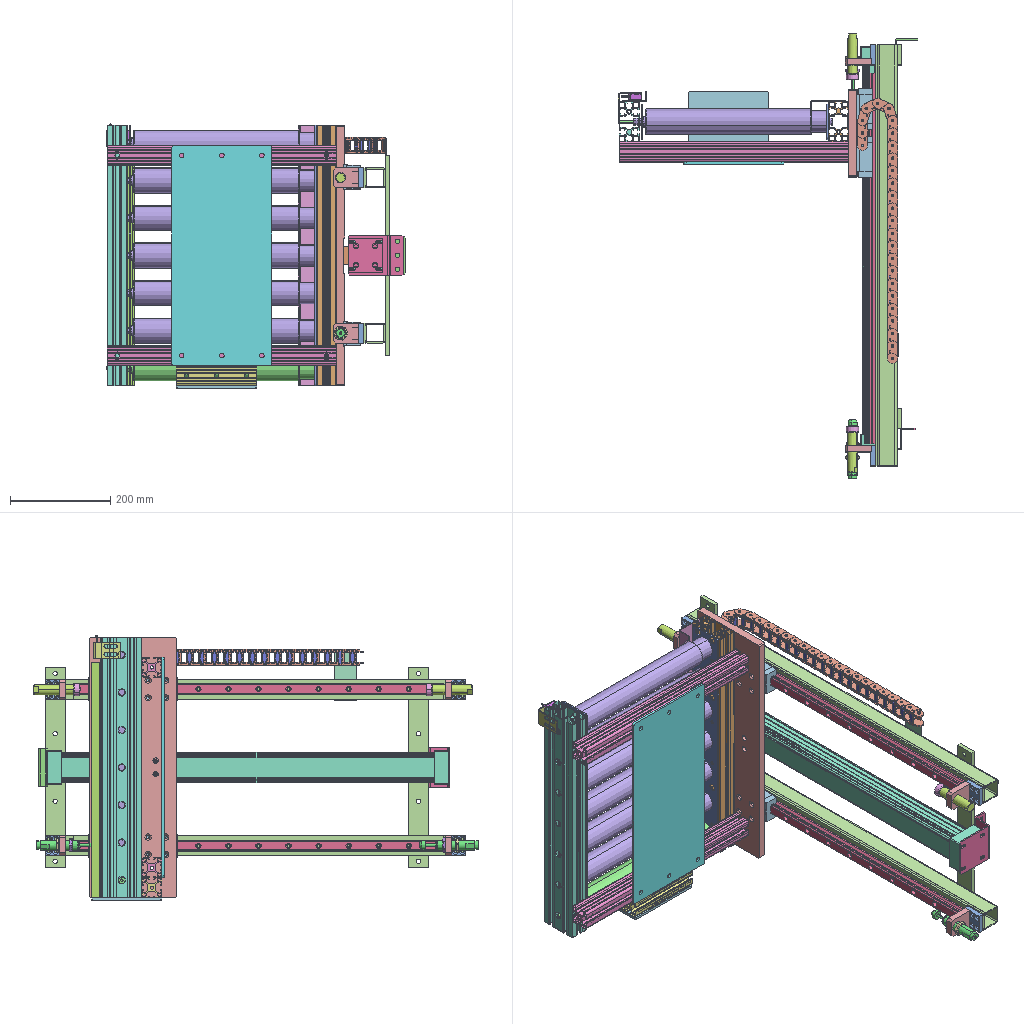Assembly | STEP file | 32 different items | 105 placed | box 598 x 888 x 528 mm
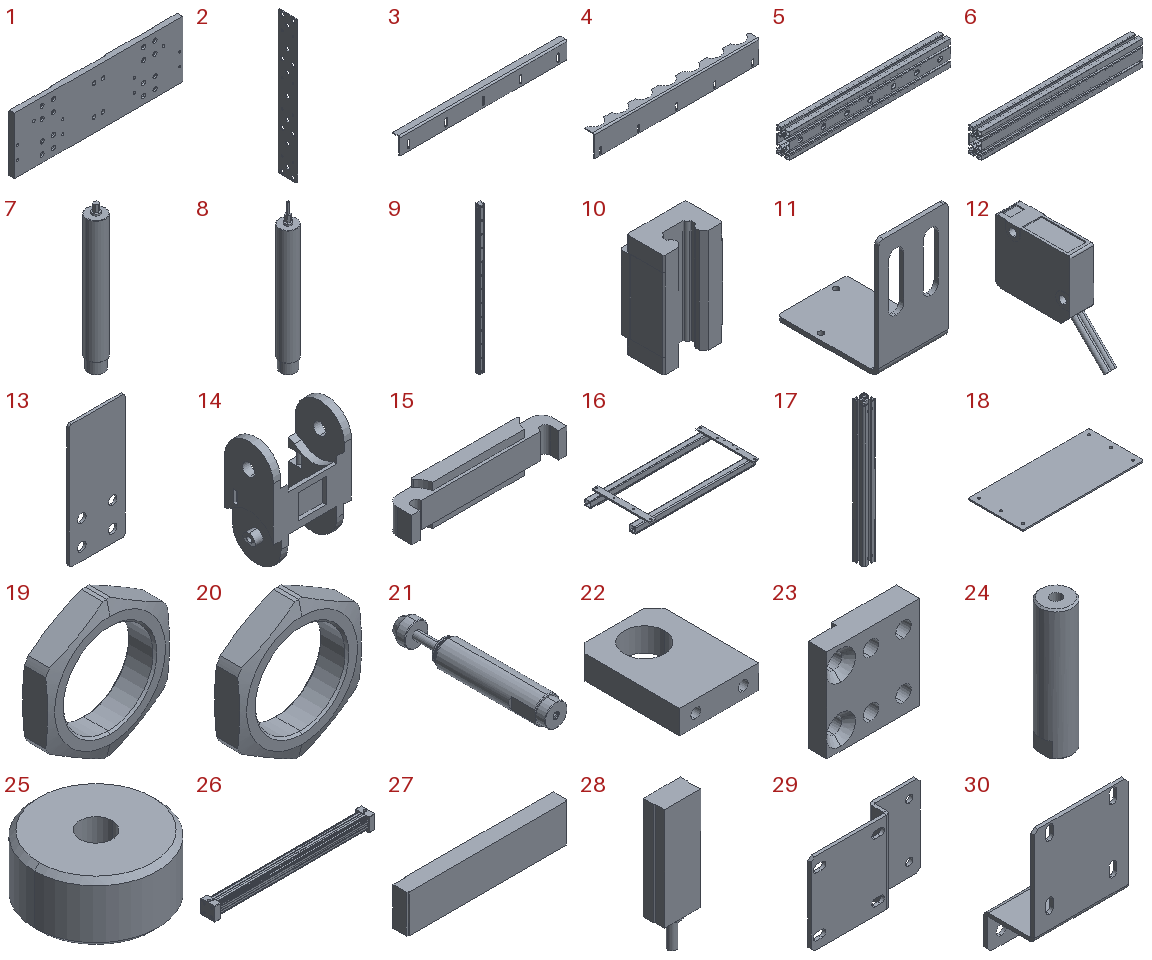Parts list (item | name | quantity | parent item | size | volume):
1 | - | x1 | - | 520 x 16 x 175 mm | 1376606 mm3
2 | - | x2 | - | 3 x 70 x 520 mm | 101913 mm3
3 | - | x1 | - | 470 x 20 x 48 mm | 59388 mm3
4 | - | x1 | - | 520 x 30 x 70 mm | 90245 mm3
5 | - | x1 | - | 520 x 40 x 80 mm | 382140 mm3
6 | - | x1 | - | 520 x 40 x 80 mm | 378549 mm3
7 | Unpowered Roller_Default | x6 | - | 50.6 x 50.6 x 396 mm | 712589 mm3
8 | Motorized Roller_Default | x1 | - | 50.6 x 50.6 x 426 mm | 713178 mm3
9 | HGH25 Rail | x2 | in HGH25CA2R740Z0 | 23 x 22 x 740 mm | 310065 mm3
10 | HGH25 Slider | x4 | in HGH25CA2R740Z0 | 48 x 34.5 x 82 mm | 100220 mm3
11 | - | x1 | - | 32 x 47 x 55 mm | 5577 mm3
12 | Proximity Switch | x1 | - | 10.4 x 45.161 x 39.591 mm | 8353 mm3
13 | - | x1 | - | 45 x 2 x 100 mm | 8685 mm3
14 | MHPU203_30c | x25 | in MHPU203_30_MHPU203-30 | 32 x 20 x 45 mm | 6087 mm3
15 | MHPU203_30f | x25 | in MHPU203_30_MHPU203-30 | 27.6 x 4.5 x 7.143 mm | 492.21 mm3
16 | - | x1 | - | 840 x 400 x 53 mm | 1080937 mm3
17 | - | x2 | - | 40 x 40 x 458 mm | 262404 mm3
18 | - | x1 | - | 440 x 200 x 5 mm | 437984 mm3
19 | ACA-2020-1 | x2 | in ACA-2020 | 26 x 6 x 29.132 mm | 1676 mm3
20 | ACA-2020-2 | x2 | in ACA-2020 | 26 x 6 x 29.132 mm | 1676 mm3
21 | ACA-2020-3 | x2 | in ACA-2020 | 20 x 118 x 20 mm | 28972 mm3
22 | - | x5 | - | 40 x 53 x 12 mm | 20571 mm3
23 | - | x5 | - | 40 x 10 x 40 mm | 12395 mm3
24 | - | x2 | - | 20 x 20 x 80 mm | 24015 mm3
25 | - | x2 | - | 25 x 25 x 12 mm | 5014 mm3
26 | HI_PRU40500b | x1 | in PRF40x500-S2_0_ | 800 x 69 x 69 mm | 2639652 mm3
27 | HI_PRF40500s | x1 | in PRF40x500-S2_0_ | 152 x 14 x 36 mm | 74599 mm3
28 | HI_S-CS-95 | x2 | in PRF40x500-S2_0_ | 10.9 x 7 x 39 mm | 1983 mm3
29 | - | x1 | - | 115 x 18 x 75 mm | 27777 mm3
30 | - | x1 | - | 80 x 43 x 110 mm | 34046 mm3
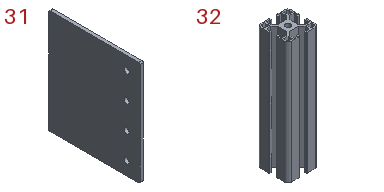31 | - | x1 | - | 5 x 140 x 160 mm | 110710 mm3
32 | - | x1 | - | 40 x 40 x 160 mm | 89766 mm3
Placements (level | parent | child | x y z in mm | rotation matrix by rows):
1 | subassembly 2 | subassembly 3 | -147.955 36.01 -80.412 | 0 1 0 0 0 -1 -1 0 0
1 | subassembly 2 | subassembly 4 | -187.955 71.51 -340.412 | -1 0 0 0 1 0 0 0 -1
1 | subassembly 2 | subassembly 4 | -558.455 71.51 -340.412 | -1 0 0 0 1 0 0 0 -1
1 | subassembly 2 | subassembly 5 | -598.455 98.51 129.588 | 0 0 1 0 1 0 -1 0 -0
1 | subassembly 2 | subassembly 6 | -154.455 100.51 179.588 | 0 0 -1 0 -1 0 -1 0 0
1 | subassembly 2 | subassembly 7 | -585.955 78.51 -340.412 | 0 1 0 0 0 1 1 0 0
1 | subassembly 2 | subassembly 8 | -167.955 38.51 -340.412 | 0 -1 0 0 0 -1 1 0 0
1 | subassembly 2 | Unpowered Roller_Default | -222.455 58.76 -230.412 | 0 0 -1 0.3439 -0.939 0 -0.939 -0.3439 0
1 | subassembly 2 | Unpowered Roller_Default | -222.455 58.76 144.588 | 0 0 -1 0.3439 -0.939 0 -0.939 -0.3439 0
1 | subassembly 2 | Unpowered Roller_Default | -222.455 58.76 69.588 | 0 0 -1 0.3439 -0.939 0 -0.939 -0.3439 0
1 | subassembly 2 | Unpowered Roller_Default | -222.455 58.76 -5.412 | 0 0 -1 0.3439 -0.939 0 -0.939 -0.3439 0
1 | subassembly 2 | Unpowered Roller_Default | -222.455 58.76 -80.412 | 0 0 -1 0.3439 -0.939 0 -0.939 -0.3439 0
1 | subassembly 2 | Unpowered Roller_Default | -222.455 58.76 -155.412 | 0 0 -1 0.3439 -0.939 0 -0.939 -0.3439 0
1 | subassembly 2 | Motorized Roller_Default | -222.455 58.361 -305.412 | 0 0 -1 0 1 0 1 0 0
1 | subassembly 2 | HGH25CA2R740Z0 | -108.387 -214.405 -232.617 | 0 -1 0 0 0 1 -1 0 -0
2 | HGH25CA2R740Z0 | HGH25 Rail | 4.046 -14.432 -225.0 | 1 0 0 0 1 0 0 0 1
2 | HGH25CA2R740Z0 | HGH25 Slider | 4.046 -14.432 297.916 | 1 0 0 0 1 0 0 0 1
2 | HGH25CA2R740Z0 | HGH25 Slider | 4.046 -14.432 202.916 | 1 0 0 0 1 0 0 0 1
1 | subassembly 2 | HGH25CA2R740Z0 | -108.387 -214.405 80.383 | 0 -1 0 0 0 1 -1 0 -0
2 | HGH25CA2R740Z0 | HGH25 Rail | 4.046 -14.432 -225.0 | 1 0 0 0 1 0 0 0 1
2 | HGH25CA2R740Z0 | HGH25 Slider | 4.046 -14.432 297.916 | 1 0 0 0 1 0 0 0 1
2 | HGH25CA2R740Z0 | HGH25 Slider | 4.046 -14.432 202.916 | 1 0 0 0 1 0 0 0 1
1 | subassembly 2 | subassembly 9 | -605.955 115.71 169.588 | 0 1 0 0 0 -1 -1 0 -0
1 | subassembly 2 | Proximity Switch | -563.955 108.51 145.388 | 0 0 1 -1 0 0 0 -1 0
1 | subassembly 2 | subassembly 10 | -47.955 -410.405 53.338 | 0 -1 0 1 0 0 0 0 1
1 | subassembly 2 | MHPU203_30_MHPU203-30 | -119.955 58.095 139.338 | 0 1 0 -1 0 0 0 0 1
2 | MHPU203_30_MHPU203-30 | MHPU203_30c | 32.5 -0.0 -0.0 | 0 0 1 0 1 0 -1 0 -0
2 | MHPU203_30_MHPU203-30 | MHPU203_30f | 10.0 -0.0 -0.0 | 0 0 1 0 1 0 -1 0 -0
2 | MHPU203_30_MHPU203-30 | MHPU203_30c | 7.067 -2.909 0.0 | 0 0.2909 0.9567 0 0.9567 -0.2909 -1 0 0
2 | MHPU203_30_MHPU203-30 | MHPU203_30f | -14.459 3.637 0.0 | 0 0.2909 0.9567 0 0.9567 -0.2909 -1 0 0
2 | MHPU203_30_MHPU203-30 | MHPU203_30c | -22.252 -1.817 -0.0 | 0 0.9091 0.4167 0 0.4167 -0.9091 -1 0 0
2 | MHPU203_30_MHPU203-30 | MHPU203_30f | -31.627 18.637 -0.0 | 0 0.9091 0.4167 0 0.4167 -0.9091 -1 0 0
2 | MHPU203_30_MHPU203-30 | MHPU203_30c | -41.002 20.909 -0.0 | 0 0.9091 -0.4167 0 -0.4167 -0.9091 -1 0 0
2 | MHPU203_30_MHPU203-30 | MHPU203_30f | -31.627 41.363 -0.0 | 0 0.9091 -0.4167 0 -0.4167 -0.9091 -1 0 0
2 | MHPU203_30_MHPU203-30 | MHPU203_30c | -35.986 49.817 -0.0 | 0 0.2909 -0.9567 0 -0.9567 -0.2909 -1 0 0
2 | MHPU203_30_MHPU203-30 | MHPU203_30f | -14.459 56.363 -0.0 | 0 0.2909 -0.9567 0 -0.9567 -0.2909 -1 0 0
2 | MHPU203_30_MHPU203-30 | MHPU203_30c | -12.5 60.0 0.0 | 0 0 -1 0 -1 0 -1 0 0
2 | MHPU203_30_MHPU203-30 | MHPU203_30f | 10 60.0 -0.0 | 0 0 -1 0 -1 0 -1 0 0
2 | MHPU203_30_MHPU203-30 | MHPU203_30c | 12.5 60.0 0.0 | 0 0 -1 0 -1 0 -1 0 0
2 | MHPU203_30_MHPU203-30 | MHPU203_30f | 35 60.0 0.0 | 0 0 -1 0 -1 0 -1 0 0
2 | MHPU203_30_MHPU203-30 | MHPU203_30c | 37.5 60.0 0.0 | 0 0 -1 0 -1 0 -1 0 0
2 | MHPU203_30_MHPU203-30 | MHPU203_30f | 60 60.0 -0.0 | 0 0 -1 0 -1 0 -1 0 0
2 | MHPU203_30_MHPU203-30 | MHPU203_30c | 62.5 60.0 -0.0 | 0 0 -1 0 -1 0 -1 0 0
2 | MHPU203_30_MHPU203-30 | MHPU203_30f | 85 60.0 -0.0 | 0 0 -1 0 -1 0 -1 0 0
2 | MHPU203_30_MHPU203-30 | MHPU203_30c | 87.5 60.0 0.0 | 0 0 -1 0 -1 0 -1 0 0
2 | MHPU203_30_MHPU203-30 | MHPU203_30f | 110 60.0 -0.0 | 0 0 -1 0 -1 0 -1 0 0
2 | MHPU203_30_MHPU203-30 | MHPU203_30f | 135 60.0 0.0 | 0 0 -1 0 -1 0 -1 0 0
2 | MHPU203_30_MHPU203-30 | MHPU203_30f | 160 60.0 -0.0 | 0 0 -1 0 -1 0 -1 0 0
2 | MHPU203_30_MHPU203-30 | MHPU203_30f | 185 60.0 -0.0 | 0 0 -1 0 -1 0 -1 0 0
2 | MHPU203_30_MHPU203-30 | MHPU203_30f | 210 60.0 -0.0 | 0 0 -1 0 -1 0 -1 0 0
2 | MHPU203_30_MHPU203-30 | MHPU203_30f | 235 60.0 0.0 | 0 0 -1 0 -1 0 -1 0 0
2 | MHPU203_30_MHPU203-30 | MHPU203_30f | 260 60.0 0.0 | 0 0 -1 0 -1 0 -1 0 0
2 | MHPU203_30_MHPU203-30 | MHPU203_30f | 285 60.0 0.0 | 0 0 -1 0 -1 0 -1 0 0
2 | MHPU203_30_MHPU203-30 | MHPU203_30f | 310 60.0 0.0 | 0 0 -1 0 -1 0 -1 0 0
2 | MHPU203_30_MHPU203-30 | MHPU203_30f | 335 60.0 -0.0 | 0 0 -1 0 -1 0 -1 0 0
2 | MHPU203_30_MHPU203-30 | MHPU203_30c | 112.5 60.0 -0.0 | 0 0 -1 0 -1 0 -1 0 0
2 | MHPU203_30_MHPU203-30 | MHPU203_30c | 137.5 60.0 0.0 | 0 0 -1 0 -1 0 -1 0 0
2 | MHPU203_30_MHPU203-30 | MHPU203_30c | 162.5 60.0 -0.0 | 0 0 -1 0 -1 0 -1 0 0
2 | MHPU203_30_MHPU203-30 | MHPU203_30c | 187.5 60.0 -0.0 | 0 0 -1 0 -1 0 -1 0 0
2 | MHPU203_30_MHPU203-30 | MHPU203_30c | 212.5 60.0 0.0 | 0 0 -1 0 -1 0 -1 0 0
2 | MHPU203_30_MHPU203-30 | MHPU203_30c | 237.5 60.0 0.0 | 0 0 -1 0 -1 0 -1 0 0
2 | MHPU203_30_MHPU203-30 | MHPU203_30c | 262.5 60.0 -0.0 | 0 0 -1 0 -1 0 -1 0 0
2 | MHPU203_30_MHPU203-30 | MHPU203_30c | 287.5 60.0 0.0 | 0 0 -1 0 -1 0 -1 0 0
2 | MHPU203_30_MHPU203-30 | MHPU203_30c | 312.5 60.0 0.0 | 0 0 -1 0 -1 0 -1 0 0
2 | MHPU203_30_MHPU203-30 | MHPU203_30c | 57.5 -0.0 -0.0 | 0 0 1 0 1 0 -1 0 -0
2 | MHPU203_30_MHPU203-30 | MHPU203_30f | 35.0 -0.0 0.0 | 0 0 1 0 1 0 -1 0 -0
2 | MHPU203_30_MHPU203-30 | MHPU203_30c | 337.5 60.0 0.0 | 0 0 -1 0 -1 0 -1 0 0
2 | MHPU203_30_MHPU203-30 | MHPU203_30c | 362.5 60.0 -0.0 | 0 0 -1 0 -1 0 -1 0 0
2 | MHPU203_30_MHPU203-30 | MHPU203_30c | 387.5 60.0 0.0 | 0 0 -1 0 -1 0 -1 0 0
2 | MHPU203_30_MHPU203-30 | MHPU203_30c | 412.5 60.0 -0.0 | 0 0 -1 0 -1 0 -1 0 0
2 | MHPU203_30_MHPU203-30 | MHPU203_30c | 437.5 60.0 0.0 | 0 0 -1 0 -1 0 -1 0 0
2 | MHPU203_30_MHPU203-30 | MHPU203_30f | 360 60.0 0.0 | 0 0 -1 0 -1 0 -1 0 0
2 | MHPU203_30_MHPU203-30 | MHPU203_30f | 385 60.0 -0.0 | 0 0 -1 0 -1 0 -1 0 0
2 | MHPU203_30_MHPU203-30 | MHPU203_30f | 410 60.0 0.0 | 0 0 -1 0 -1 0 -1 0 0
2 | MHPU203_30_MHPU203-30 | MHPU203_30f | 435 60.0 0.0 | 0 0 -1 0 -1 0 -1 0 0
2 | MHPU203_30_MHPU203-30 | MHPU203_30f | 460 60.0 -0.0 | 0 0 -1 0 -1 0 -1 0 0
1 | subassembly 2 | subassembly 11 | -70.955 -628.405 -235.162 | 0 0 1 1 0 0 0 1 -0
1 | subassembly 2 | subassembly 12 | -147.955 -1.49 -280.412 | 0 0 1 0 1 0 -1 0 -0
1 | subassembly 2 | subassembly 12 | -147.955 -1.49 119.588 | 0 0 1 0 1 0 -1 0 -0
1 | subassembly 2 | subassembly 13 | -476.955 -26.49 -300.412 | 0 1 0 0 0 1 1 0 -0
1 | subassembly 2 | ACA-2020 | -139.955 -653.405 -235.162 | -0.9745 0 0.2243 0 1 0 -0.2243 0 -0.9745
2 | ACA-2020 | ACA-2020-1 | -0.0 -22.0 -0.0 | 0.9939 0 -0.11 0 1 0 0.11 0 0.9939
2 | ACA-2020 | ACA-2020-2 | -0.0 -2.0 -0.0 | 0.9756 0 0.2198 0 1 0 -0.2198 0 0.9756
2 | ACA-2020 | ACA-2020-3 | -0.0 -0.0 -0.0 | 1 0 0 0 1 0 0 0 1
1 | subassembly 2 | subassembly 14 | -101.955 -588.405 -255.162 | 0 -1 0 0 0 -1 1 0 -0
1 | subassembly 2 | subassembly 15 | -93.955 -588.405 -215.162 | 0 -1 0 -1 0 0 0 0 -1
1 | subassembly 2 | subassembly 15 | -93.955 171.595 -255.162 | 0 -1 0 1 0 0 0 0 1
1 | subassembly 2 | subassembly 14 | -101.955 183.595 -255.162 | 0 -1 0 0 0 -1 1 0 0
1 | subassembly 2 | ACA-2020 | -139.955 228.595 -235.162 | 0.9385 0 0.3453 0 -1 0 0.3453 0 -0.9385
2 | ACA-2020 | ACA-2020-1 | -0.0 -22.0 -0.0 | 0.9939 0 -0.11 0 1 0 0.11 0 0.9939
2 | ACA-2020 | ACA-2020-2 | -0.0 -2.0 -0.0 | 0.9756 0 0.2198 0 1 0 -0.2198 0 0.9756
2 | ACA-2020 | ACA-2020-3 | -0.0 -0.0 -0.0 | 1 0 0 0 1 0 0 0 1
1 | subassembly 2 | subassembly 15 | -93.955 171.595 54.838 | 0 -1 0 1 0 0 0 0 1
1 | subassembly 2 | subassembly 14 | -101.955 183.595 54.838 | 0 -1 0 0 0 -1 1 0 0
1 | subassembly 2 | subassembly 16 | -139.955 234.595 74.838 | 1 0 0 0 0 -1 0 1 -0
1 | subassembly 2 | subassembly 16 | -139.955 -641.405 74.838 | 0.8372 0.5469 0 0 0 1 0.5469 -0.8372 -0
1 | subassembly 2 | subassembly 17 | -139.955 142.595 74.838 | 0.9237 0.383 0 0 0 1 0.383 -0.9237 0
1 | subassembly 2 | subassembly 17 | -139.955 -549.405 74.838 | 1 0 0 0 0 -1 0 1 0
1 | subassembly 2 | subassembly 14 | -101.955 -588.405 54.838 | 0 -1 0 0 0 -1 1 0 -0
1 | subassembly 2 | subassembly 15 | -93.955 -588.405 94.838 | 0 -1 0 -1 0 0 0 0 -1
1 | subassembly 2 | subassembly 15 | -93.955 171.595 54.838 | 0 -1 0 1 0 0 0 0 1
1 | subassembly 2 | subassembly 14 | -101.955 183.595 54.838 | 0 -1 0 0 0 -1 1 0 0
1 | subassembly 2 | PRF40x500-S2_0_ | -61.701 185.013 -59.225 | 0 -1 0 0 0 1 -1 0 0
2 | PRF40x500-S2_0_ | HI_PRU40500b | 20.938 -6.247 21.581 | 0 0 1 0 1 0 -1 0 0
2 | PRF40x500-S2_0_ | HI_PRF40500s | 20.938 58.253 -149.003 | 0 0 -1 0 1 0 1 0 -0
2 | PRF40x500-S2_0_ | HI_S-CS-95 | 28.1 35.4 -2.5 | 0 1 0 -1 0 0 0 0 1
2 | PRF40x500-S2_0_ | HI_S-CS-95 | 28.1 35.4 -741.5 | 0 1 0 1 0 0 0 0 -1
1 | subassembly 2 | subassembly 18 | -124.455 209.595 -117.662 | 1 0 0 0 1 0 0 0 1
1 | subassembly 2 | subassembly 19 | -124.455 -593.405 -120.162 | 0 0 -1 0 1 0 1 0 0
1 | subassembly 2 | subassembly 20 | -467.455 -21.339 -340.412 | 0 0 1 0 1 0 -1 0 -0
1 | subassembly 2 | subassembly 21 | -307.455 -1.49 -320.412 | 0 0 1 1 0 0 0 1 -0